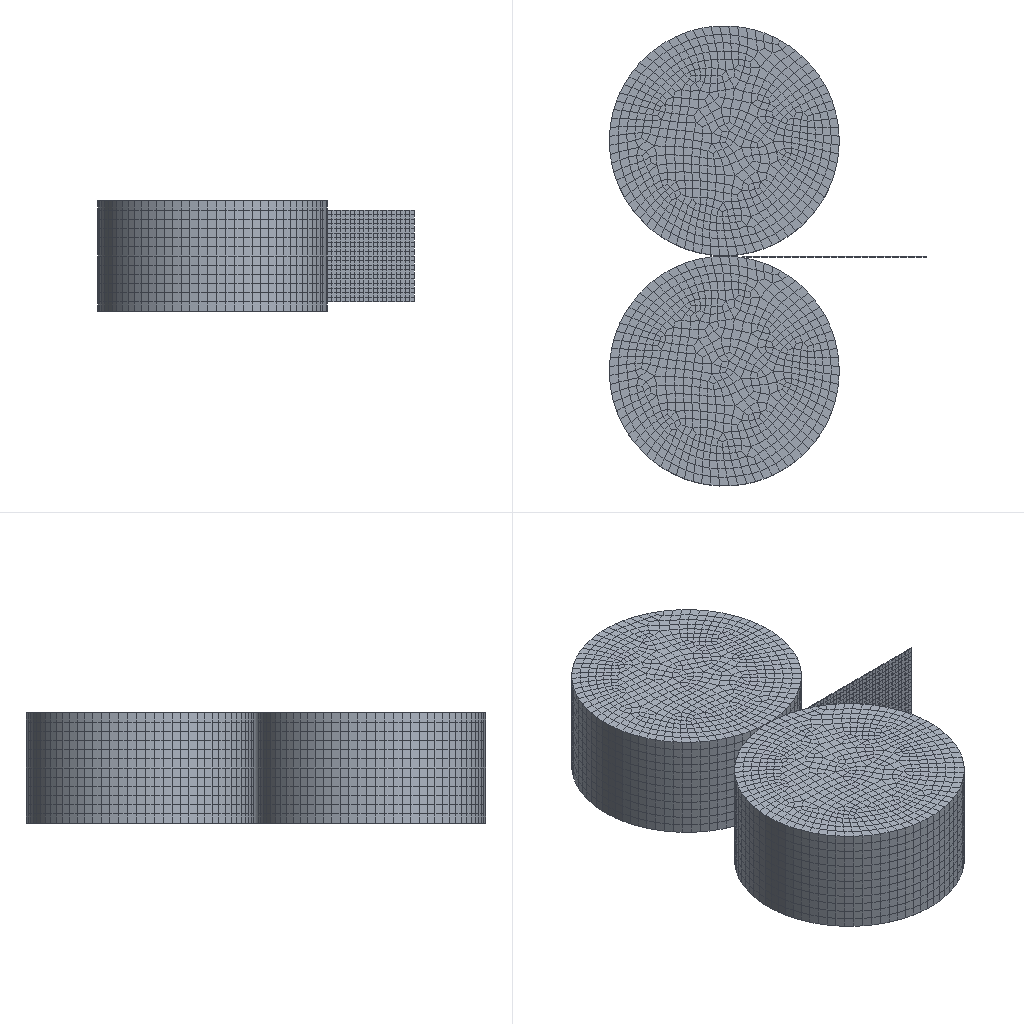Simulation study | abaqus
Set-up summary:
category,name,step,type,value,unit,region
solver,abaqus
solver,version,,,Abaqus/Explicit 2020
units,not stated in the deck,,not stated
analysis,deck,,dynamic temperature-displacement,dynamic temperature-displacement
load_step,Step-1,Step-1,dynamic temperature-displacement
load_step,requested,,,1
mesh,nodes,,,20988
mesh,elements,,,17600
element_type,C3D8RT,,solid,17600
load,load commands in deck,,count,3
bc,support commands in deck,,count,3
material,MATERIAL-1,,in results
material,RIG,,in results
check,setup vs results,,match,"per instance, exact: element labels, types and connectivity; labels of the nodes the elements use; coordinates of those nodes at SINGLE_PRECISION in 3 of 3 instance(s)"
Abaqus input file, long lists of numbers shortened:
*Heading
** Job name: Job-1 Model name: Model-1
** Generated by: Abaqus/CAE 2020
*Preprint, echo=NO, model=NO, history=NO, contact=NO
**
** PARTS
**
*Part, name=rig
*Node
      1,   77.43,  -98.131,           0.
      2,   98.199,  -77.344,           0.
** (9631 more lines like these left out)
*Element, type=C3D8RT
   1,  868,  820,  769,  905,  127,   79,   28,  164
   2,  866,  818,  768, 1365,  125,   77,   27,  624
** (8398 more lines like these left out)
*Nset, nset=Set-1, generate
    1,  9633,     1
*Elset, elset=Set-1, generate
    1,  8400,     1
** Section: rig
*Solid Section, elset=Set-1, material=rig
,
*End Part
**
*Part, name=work
*Node
      1,           0.,        -100.,           1.
      2,           0.,         -95.,           1.
** (1720 more lines like these left out)
*Element, type=C3D8RT
  1,   43,   44,   65,   64,    1,    2,   23,   22
  2,   44,   45,   66,   65,    2,    3,   24,   23
** (798 more lines like these left out)
*Nset, nset=Set-1, generate
    1,  1722,     1
*Elset, elset=Set-1, generate
   1,  800,    1
** Section: Section-1
*Solid Section, elset=Set-1, material=Material-1
,
*End Part
**
**
** ASSEMBLY
**
*Assembly, name=Assembly
**
*Instance, name=rig-1, part=rig
          0.,         125.,        -110.
*End Instance
**
*Instance, name=work-1, part=work
         20.,         -0.4,           0.
         20.,         -0.4,           0., 21.,         -0.4,           0., 90.
*End Instance
**
*Instance, name=rig-1-lin-2-1, part=rig
          0.,       -125.6,        -110.
*End Instance
**
*Node
      1,           0.,         125.,          10.
*Node
      2,           0.,  -125.6,          10.
*Nset, nset=Set-5
 1, 2
*Nset, nset=Set-6, instance=work-1, generate
 1681,  1722,     1
*Elset, elset=Set-6, instance=work-1, generate
 781,  800,    1
*Nset, nset=Set-7, instance=work-1, generate
  1,  42,   1
*Elset, elset=Set-7, instance=work-1, generate
  1,  20,   1
*Nset, nset=Set-8, instance=work-1, generate
 1681,  1722,     1
*Elset, elset=Set-8, instance=work-1, generate
 781,  800,    1
*Nset, nset=Set-9, instance=work-1, generate
    1,  1722,     1
*Elset, elset=Set-9, instance=work-1, generate
   1,  800,    1
*Nset, nset=b_Set-1, instance=rig-1, generate
    1,  9633,     1
*Elset, elset=b_Set-1, instance=rig-1, generate
    1,  8400,     1
*Nset, nset=b_Set-3, instance=rig-1-lin-2-1, generate
    1,  9633,     1
*Elset, elset=b_Set-3, instance=rig-1-lin-2-1, generate
    1,  8400,     1
*Nset, nset=_PickedSet11, internal
 1,
*Nset, nset=_PickedSet13, internal
 2,
*Elset, elset=_Surf-5_S1, internal, instance=work-1, generate
 781,  800,    1
*Elset, elset=_Surf-5_S6, internal, instance=work-1, generate
   1,  781,   20
*Elset, elset=_Surf-5_S2, internal, instance=work-1, generate
  1,  20,   1
*Elset, elset=_Surf-5_S4, internal, instance=work-1, generate
  20,  800,   20
*Elset, elset=_Surf-5_S3, internal, instance=work-1, generate
   1,  800,    1
*Elset, elset=_Surf-5_S5, internal, instance=work-1, generate
   1,  800,    1
*Surface, type=ELEMENT, name=Surf-5
_Surf-5_S1, S1
_Surf-5_S6, S6
_Surf-5_S2, S2
_Surf-5_S4, S4
_Surf-5_S3, S3
_Surf-5_S5, S5
*Elset, elset=_Surf-6_S1, internal, instance=work-1, generate
 781,  800,    1
*Elset, elset=_Surf-6_S2, internal, instance=work-1, generate
  1,  20,   1
*Surface, type=ELEMENT, name=Surf-6
_Surf-6_S1, S1
_Surf-6_S2, S2
*Elset, elset=_m_Surf-1_S4, internal, instance=rig-1
    1,    2,    4,    5,    8,   14,   16,   21,   24,   28,   29,   32,   33,   35,   36,   37
   38,   41,   42,   43,   49,   54,   59,   63,   69,   70,   71,   72,   73,   74,   75,   77
** (31 more lines like these left out)
*Elset, elset=_m_Surf-1_S6, internal, instance=rig-1
    3,    6,    7,    9,   10,   11,   12,   13,   17,   18,   20,   22,   30,   34,   39,   46
   48,   50,   52,   55,   56,   57,   60,   61,   62,   65,   66,   67,   68,   76,   90,   96
** (25 more lines like these left out)
*Surface, type=ELEMENT, name=m_Surf-1
_m_Surf-1_S4, S4
_m_Surf-1_S6, S6
*Elset, elset=_m_Surf-3_S4, internal, instance=rig-1-lin-2-1
    1,    2,    4,    5,    8,   14,   16,   21,   24,   28,   29,   32,   33,   35,   36,   37
   38,   41,   42,   43,   49,   54,   59,   63,   69,   70,   71,   72,   73,   74,   75,   77
** (31 more lines like these left out)
*Elset, elset=_m_Surf-3_S6, internal, instance=rig-1-lin-2-1
    3,    6,    7,    9,   10,   11,   12,   13,   17,   18,   20,   22,   30,   34,   39,   46
   48,   50,   52,   55,   56,   57,   60,   61,   62,   65,   66,   67,   68,   76,   90,   96
** (25 more lines like these left out)
*Surface, type=ELEMENT, name=m_Surf-3
_m_Surf-3_S4, S4
_m_Surf-3_S6, S6
*Elset, elset=_s_Surf-1_S5, internal, instance=work-1, generate
   1,  800,    1
*Surface, type=ELEMENT, name=s_Surf-1
_s_Surf-1_S5, S5
*Elset, elset=_s_Surf-3_S3, internal, instance=work-1, generate
   1,  800,    1
*Surface, type=ELEMENT, name=s_Surf-3
_s_Surf-3_S3, S3
** Constraint: Constraint-1
*Rigid Body, ref node=_PickedSet11, elset=b_Set-1
** Constraint: Constraint-2
*Rigid Body, ref node=_PickedSet13, elset=b_Set-3
*End Assembly
*Amplitude, name=Amp-1
             0.,              0.,            0.01,              1.
**
** MATERIALS
**
*Material, name=Material-1
*Conductivity
155.,
*Density
 2.5e-09,
*Elastic
45000., 0.308
*Expansion
 2e-05,
*Plastic
 33.,    0.
 60., 0.017
 85., 0.026
105., 0.034
121., 0.043
136., 0.052
150.,  0.06
165.,  0.07
200., 0.094
230.,  0.12
240., 0.142
*Specific Heat
 9e+08,
*Material, name=rig
*Conductivity
45.,
*Density
 7.8e-09,
*Elastic
210000., 0.3
*Specific Heat
 4.6e+08,
**
** INTERACTION PROPERTIES
**
*Surface Interaction, name=IntProp-1
*Friction
 0.15,
*Surface Behavior, pressure-overclosure=HARD
*Gap Conductance
11.,   0.
 0., 0.01
** ----------------------------------------------------------------
**
** STEP: Step-1
**
*Step, name=Step-1, nlgeom=YES
*Dynamic Temperature-displacement, Explicit
, 0.01
*Bulk Viscosity
0.06, 1.2
**
** BOUNDARY CONDITIONS
**
** Name: BC-1 Type: 对称/反对称/完全固定
*Boundary
Set-5, ENCASTRE
** Name: [REDACTED] : Displacement/rotation angle
*Boundary, amplitude=Amp-1
Set-9, 1, 1, -300.
**
** LOADS
**
** Name: Load-1   Type: Pressure
*Dsload
Surf-6, P, -15.
**
** INTERACTIONS
**
** Interaction: Int-1
*Contact Pair, interaction=IntProp-1, mechanical constraint=KINEMATIC, cpset=Int-1
m_Surf-1, s_Surf-1
** Interaction: Int-1-Copy
*Contact Pair, interaction=IntProp-1, mechanical constraint=KINEMATIC, cpset=Int-1-Copy
m_Surf-3, s_Surf-3
** Interaction: Int-3
*Sfilm
Surf-5, F, 25., 0.016
**
** OUTPUT REQUESTS
**
*Restart, write, number interval=1, time marks=NO
**
** FIELD OUTPUT: F-Output-1
**
*Output, field, number interval=50
*Node Output
A, CF, NT, RF, RFL, RM, RT, U
V
*Element Output, directions=YES
E, EVF, HFL, LE, MISES, MISESMAX, PE, PEEQ, PEEQVAVG, PEVAVG, S, SF, SVAVG, TEMP, YIELDPOT
*Contact Output
CDISP, CSTRESS
**
** HISTORY OUTPUT: H-Output-1
**
*Output, history, variable=PRESELECT
*End Step
Results summary:
result,step,Step-1,completed,increments=71454 time=0.01/0.01
result,analysis,,,"dynamic temperature-displacement, explict"
result,last_loadstep,,,1
result,primary field,,,"U, NT11"
result,reaction total,,FX,354.898,model units
result,reaction total,,FY,0.0,model units
result,reaction total,,FZ,0.0,model units